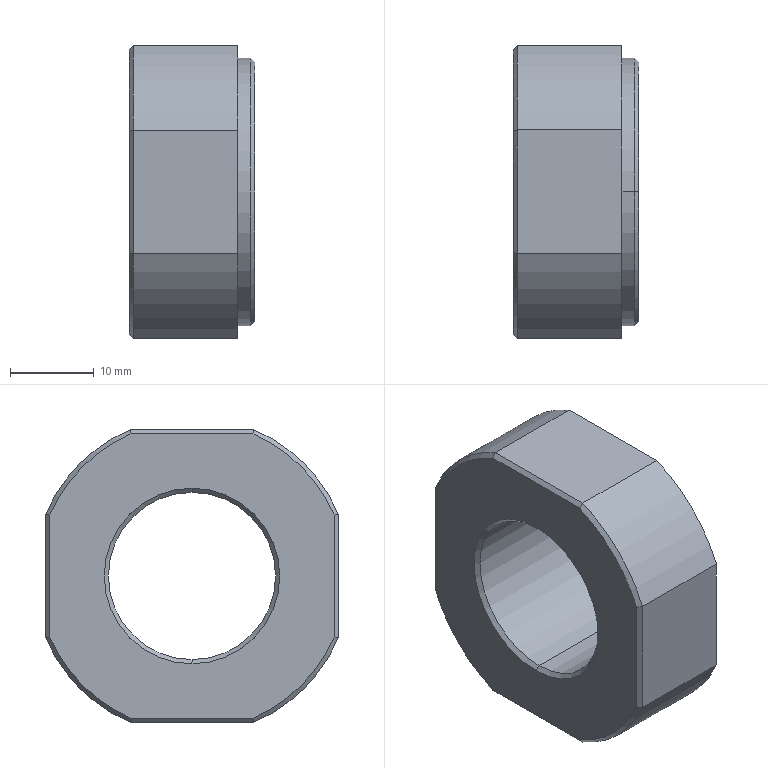Part | SolidWorks | features ICE 2, Chamfer 1, Extrusion 1 | 1 solid | 29 faces | box 15 x 35 x 35 mm | volume 10821 mm3 | plane 11 | cone 10 | cylinder 8 | commonest cylinder face diameters 38 x4 20 x2 32 x2
STEP:
#1=CARTESIAN_POINT('',(14.5,0.,10.));
#2=VERTEX_POINT('',#1);
#3=CARTESIAN_POINT('',(14.5,0.,-10.));
#4=VERTEX_POINT('',#3);
#5=CARTESIAN_POINT('',(14.5,0.,0.));
#6=DIRECTION('',(1.,0.,0.));
#7=DIRECTION('',(0.,0.,-1.));
#8=AXIS2_PLACEMENT_3D('',#5,#6,#7);
#9=CIRCLE('',#8,10.);
#10=EDGE_CURVE('',#2,#4,#9,.T.);
#11=ORIENTED_EDGE('',*,*,#10,.F.);
#12=CARTESIAN_POINT('',(15.,0.,10.5));
#13=VERTEX_POINT('',#12);
#14=CARTESIAN_POINT('',(14.5,0.,10.));
#15=DIRECTION('',(0.7071,0.,0.7071));
#16=VECTOR('',#15,1000.);
#17=LINE('',#14,#16);
#18=EDGE_CURVE('',#2,#13,#17,.T.);
#19=ORIENTED_EDGE('',*,*,#18,.T.);
#20=CARTESIAN_POINT('',(15.,0.,-10.5));
#21=VERTEX_POINT('',#20);
#22=CARTESIAN_POINT('',(15.,0.,0.));
#23=DIRECTION('',(-1.,0.,0.));
#24=DIRECTION('',(0.,0.,-1.));
#25=AXIS2_PLACEMENT_3D('',#22,#23,#24);
#26=CIRCLE('',#25,10.5);
#27=EDGE_CURVE('',#21,#13,#26,.T.);
#28=ORIENTED_EDGE('',*,*,#27,.F.);
#29=CARTESIAN_POINT('',(14.5,0.,-10.));
#30=DIRECTION('',(0.7071,0.,-0.7071));
#31=VECTOR('',#30,1000.);
#32=LINE('',#29,#31);
#33=EDGE_CURVE('',#4,#21,#32,.T.);
#34=ORIENTED_EDGE('',*,*,#33,.F.);
#35=EDGE_LOOP('',(#11,#19,#28,#34));
#36=FACE_OUTER_BOUND('',#35,.T.);
#37=CARTESIAN_POINT('',(14.5,0.,0.));
#38=DIRECTION('',(1.,0.,0.));
#39=DIRECTION('',(0.,0.,-1.));
#40=AXIS2_PLACEMENT_3D('',#37,#38,#39);
#41=CONICAL_SURFACE('',#40,10.,0.7854);
#42=ADVANCED_FACE('',(#36),#41,.F.);
#43=CARTESIAN_POINT('',(15.,0.,-15.5));
#44=VERTEX_POINT('',#43);
#45=CARTESIAN_POINT('',(15.,0.,15.5));
#46=VERTEX_POINT('',#45);
#47=CARTESIAN_POINT('',(15.,0.,0.));
#48=DIRECTION('',(1.,0.,0.));
#49=DIRECTION('',(0.,0.,-1.));
#50=AXIS2_PLACEMENT_3D('',#47,#48,#49);
#51=CIRCLE('',#50,15.5);
#52=EDGE_CURVE('',#44,#46,#51,.T.);
#53=ORIENTED_EDGE('',*,*,#52,.F.);
#54=CARTESIAN_POINT('',(14.5,0.,-16.));
#55=VERTEX_POINT('',#54);
#56=CARTESIAN_POINT('',(15.,0.,-15.5));
#57=DIRECTION('',(-0.7071,0.,-0.7071));
#58=VECTOR('',#57,1000.);
#59=LINE('',#56,#58);
#60=EDGE_CURVE('',#44,#55,#59,.T.);
#61=ORIENTED_EDGE('',*,*,#60,.T.);
#62=CARTESIAN_POINT('',(14.5,0.,16.));
#63=VERTEX_POINT('',#62);
#64=CARTESIAN_POINT('',(14.5,0.,0.));
#65=DIRECTION('',(-1.,0.,0.));
#66=DIRECTION('',(0.,0.,-1.));
#67=AXIS2_PLACEMENT_3D('',#64,#65,#66);
#68=CIRCLE('',#67,16.);
#69=EDGE_CURVE('',#63,#55,#68,.T.);
#70=ORIENTED_EDGE('',*,*,#69,.F.);
#71=CARTESIAN_POINT('',(15.,0.,15.5));
#72=DIRECTION('',(-0.7071,0.,0.7071));
#73=VECTOR('',#72,1000.);
#74=LINE('',#71,#73);
#75=EDGE_CURVE('',#46,#63,#74,.T.);
#76=ORIENTED_EDGE('',*,*,#75,.F.);
#77=EDGE_LOOP('',(#53,#61,#70,#76));
#78=FACE_OUTER_BOUND('',#77,.T.);
#79=CARTESIAN_POINT('',(15.,0.,0.));
#80=DIRECTION('',(-1.,0.,0.));
#81=DIRECTION('',(0.,0.,1.));
#82=AXIS2_PLACEMENT_3D('',#79,#80,#81);
#83=CONICAL_SURFACE('',#82,15.5,0.7854);
#84=ADVANCED_FACE('',(#78),#83,.T.);
#85=CARTESIAN_POINT('',(0.5,0.,-10.));
#86=VERTEX_POINT('',#85);
#87=CARTESIAN_POINT('',(0.5,0.,10.));
#88=VERTEX_POINT('',#87);
#89=CARTESIAN_POINT('',(0.5,0.,0.));
#90=DIRECTION('',(-1.,0.,0.));
#91=DIRECTION('',(0.,0.,-1.));
#92=AXIS2_PLACEMENT_3D('',#89,#90,#91);
#93=CIRCLE('',#92,10.);
#94=EDGE_CURVE('',#86,#88,#93,.T.);
#95=ORIENTED_EDGE('',*,*,#94,.F.);
#96=CARTESIAN_POINT('',(0.,0.,-10.5));
#97=VERTEX_POINT('',#96);
#98=CARTESIAN_POINT('',(0.,0.,-10.5));
#99=DIRECTION('',(-0.7071,0.,-0.7071));
#100=VECTOR('',#99,1000.);
#101=LINE('',#98,#100);
#102=EDGE_CURVE('',#86,#97,#101,.T.);
#103=ORIENTED_EDGE('',*,*,#102,.T.);
#104=CARTESIAN_POINT('',(0.,0.,10.5));
#105=VERTEX_POINT('',#104);
#106=CARTESIAN_POINT('',(0.,0.,0.));
#107=DIRECTION('',(1.,0.,0.));
#108=DIRECTION('',(0.,0.,-1.));
#109=AXIS2_PLACEMENT_3D('',#106,#107,#108);
#110=CIRCLE('',#109,10.5);
#111=EDGE_CURVE('',#105,#97,#110,.T.);
#112=ORIENTED_EDGE('',*,*,#111,.F.);
#113=CARTESIAN_POINT('',(0.,0.,10.5));
#114=DIRECTION('',(-0.7071,0.,0.7071));
#115=VECTOR('',#114,1000.);
#116=LINE('',#113,#115);
#117=EDGE_CURVE('',#88,#105,#116,.T.);
#118=ORIENTED_EDGE('',*,*,#117,.F.);
#119=EDGE_LOOP('',(#95,#103,#112,#118));
#120=FACE_OUTER_BOUND('',#119,.T.);
#121=CARTESIAN_POINT('',(0.,0.,0.));
#122=DIRECTION('',(-1.,0.,0.));
#123=DIRECTION('',(0.,0.,1.));
#124=AXIS2_PLACEMENT_3D('',#121,#122,#123);
#125=CONICAL_SURFACE('',#124,10.5,0.7854);
#126=ADVANCED_FACE('',(#120),#125,.F.);
#127=CARTESIAN_POINT('',(13.,0.,-16.));
#128=VERTEX_POINT('',#127);
#129=CARTESIAN_POINT('',(13.,0.,16.));
#130=VERTEX_POINT('',#129);
#131=CARTESIAN_POINT('',(13.,0.,0.));
#132=DIRECTION('',(1.,0.,0.));
#133=DIRECTION('',(0.,0.,-1.));
#134=AXIS2_PLACEMENT_3D('',#131,#132,#133);
#135=CIRCLE('',#134,16.);
#136=EDGE_CURVE('',#128,#130,#135,.T.);
#137=ORIENTED_EDGE('',*,*,#136,.T.);
#138=CARTESIAN_POINT('',(13.,0.,16.));
#139=DIRECTION('',(1.,0.,0.));
#140=VECTOR('',#139,1000.);
#141=LINE('',#138,#140);
#142=EDGE_CURVE('',#130,#63,#141,.T.);
#143=ORIENTED_EDGE('',*,*,#142,.T.);
#144=ORIENTED_EDGE('',*,*,#69,.T.);
#145=CARTESIAN_POINT('',(13.,0.,-16.));
#146=DIRECTION('',(1.,0.,0.));
#147=VECTOR('',#146,1000.);
#148=LINE('',#145,#147);
#149=EDGE_CURVE('',#128,#55,#148,.T.);
#150=ORIENTED_EDGE('',*,*,#149,.F.);
#151=EDGE_LOOP('',(#137,#143,#144,#150));
#152=FACE_OUTER_BOUND('',#151,.T.);
#153=CARTESIAN_POINT('',(13.,0.,0.));
#154=DIRECTION('',(1.,0.,0.));
#155=DIRECTION('',(0.,0.,-1.));
#156=AXIS2_PLACEMENT_3D('',#153,#154,#155);
#157=CYLINDRICAL_SURFACE('',#156,16.);
#158=ADVANCED_FACE('',(#152),#157,.T.);
#159=ORIENTED_EDGE('',*,*,#10,.T.);
#160=CARTESIAN_POINT('',(15.,0.,-10.));
#161=DIRECTION('',(-1.,0.,0.));
#162=VECTOR('',#161,1000.);
#163=LINE('',#160,#162);
#164=EDGE_CURVE('',#4,#86,#163,.T.);
#165=ORIENTED_EDGE('',*,*,#164,.T.);
#166=ORIENTED_EDGE('',*,*,#94,.T.);
#167=CARTESIAN_POINT('',(15.,0.,10.));
#168=DIRECTION('',(-1.,0.,0.));
#169=VECTOR('',#168,1000.);
#170=LINE('',#167,#169);
#171=EDGE_CURVE('',#2,#88,#170,.T.);
#172=ORIENTED_EDGE('',*,*,#171,.F.);
#173=EDGE_LOOP('',(#159,#165,#166,#172));
#174=FACE_OUTER_BOUND('',#173,.T.);
#175=CARTESIAN_POINT('',(15.,0.,0.));
#176=DIRECTION('',(-1.,0.,0.));
#177=DIRECTION('',(0.,0.,1.));
#178=AXIS2_PLACEMENT_3D('',#175,#176,#177);
#179=CYLINDRICAL_SURFACE('',#178,10.);
#180=ADVANCED_FACE('',(#174),#179,.F.);
#181=CARTESIAN_POINT('',(0.5,17.5,7.399));
#182=VERTEX_POINT('',#181);
#183=CARTESIAN_POINT('',(13.,17.5,7.399));
#184=VERTEX_POINT('',#183);
#185=CARTESIAN_POINT('',(15.,17.5,7.399));
#186=DIRECTION('',(1.,0.,0.));
#187=VECTOR('',#186,1000.);
#188=LINE('',#185,#187);
#189=EDGE_CURVE('',#182,#184,#188,.T.);
#190=ORIENTED_EDGE('',*,*,#189,.F.);
#191=CARTESIAN_POINT('',(0.5,7.399,17.5));
#192=VERTEX_POINT('',#191);
#193=CARTESIAN_POINT('',(0.5,0.,0.));
#194=DIRECTION('',(1.,0.,0.));
#195=DIRECTION('',(0.,0.,-1.));
#196=AXIS2_PLACEMENT_3D('',#193,#194,#195);
#197=CIRCLE('',#196,19.);
#198=EDGE_CURVE('',#182,#192,#197,.T.);
#199=ORIENTED_EDGE('',*,*,#198,.T.);
#200=CARTESIAN_POINT('',(13.,7.399,17.5));
#201=VERTEX_POINT('',#200);
#202=CARTESIAN_POINT('',(15.,7.399,17.5));
#203=DIRECTION('',(-1.,0.,0.));
#204=VECTOR('',#203,1000.);
#205=LINE('',#202,#204);
#206=EDGE_CURVE('',#201,#192,#205,.T.);
#207=ORIENTED_EDGE('',*,*,#206,.F.);
#208=CARTESIAN_POINT('',(13.,0.,0.));
#209=DIRECTION('',(1.,0.,0.));
#210=DIRECTION('',(0.,0.,-1.));
#211=AXIS2_PLACEMENT_3D('',#208,#209,#210);
#212=CIRCLE('',#211,19.);
#213=EDGE_CURVE('',#184,#201,#212,.T.);
#214=ORIENTED_EDGE('',*,*,#213,.F.);
#215=EDGE_LOOP('',(#190,#199,#207,#214));
#216=FACE_OUTER_BOUND('',#215,.T.);
#217=CARTESIAN_POINT('',(15.,0.,0.));
#218=DIRECTION('',(-1.,0.,0.));
#219=DIRECTION('',(0.,0.,1.));
#220=AXIS2_PLACEMENT_3D('',#217,#218,#219);
#221=CYLINDRICAL_SURFACE('',#220,19.);
#222=ADVANCED_FACE('',(#216),#221,.T.);
#223=CARTESIAN_POINT('',(0.5,-7.399,17.5));
#224=VERTEX_POINT('',#223);
#225=CARTESIAN_POINT('',(13.,-7.399,17.5));
#226=VERTEX_POINT('',#225);
#227=CARTESIAN_POINT('',(15.,-7.399,17.5));
#228=DIRECTION('',(1.,0.,0.));
#229=VECTOR('',#228,1000.);
#230=LINE('',#227,#229);
#231=EDGE_CURVE('',#224,#226,#230,.T.);
#232=ORIENTED_EDGE('',*,*,#231,.F.);
#233=CARTESIAN_POINT('',(0.5,-17.5,7.399));
#234=VERTEX_POINT('',#233);
#235=CARTESIAN_POINT('',(0.5,0.,0.));
#236=DIRECTION('',(1.,0.,0.));
#237=DIRECTION('',(0.,0.,-1.));
#238=AXIS2_PLACEMENT_3D('',#235,#236,#237);
#239=CIRCLE('',#238,19.);
#240=EDGE_CURVE('',#224,#234,#239,.T.);
#241=ORIENTED_EDGE('',*,*,#240,.T.);
#242=CARTESIAN_POINT('',(13.,-17.5,7.399));
#243=VERTEX_POINT('',#242);
#244=CARTESIAN_POINT('',(15.,-17.5,7.399));
#245=DIRECTION('',(-1.,0.,0.));
#246=VECTOR('',#245,1000.);
#247=LINE('',#244,#246);
#248=EDGE_CURVE('',#243,#234,#247,.T.);
#249=ORIENTED_EDGE('',*,*,#248,.F.);
#250=CARTESIAN_POINT('',(13.,0.,0.));
#251=DIRECTION('',(1.,0.,0.));
#252=DIRECTION('',(0.,0.,-1.));
#253=AXIS2_PLACEMENT_3D('',#250,#251,#252);
#254=CIRCLE('',#253,19.);
#255=EDGE_CURVE('',#226,#243,#254,.T.);
#256=ORIENTED_EDGE('',*,*,#255,.F.);
#257=EDGE_LOOP('',(#232,#241,#249,#256));
#258=FACE_OUTER_BOUND('',#257,.T.);
#259=CARTESIAN_POINT('',(15.,0.,0.));
#260=DIRECTION('',(-1.,0.,0.));
#261=DIRECTION('',(0.,0.,1.));
#262=AXIS2_PLACEMENT_3D('',#259,#260,#261);
#263=CYLINDRICAL_SURFACE('',#262,19.);
#264=ADVANCED_FACE('',(#258),#263,.T.);
#265=CARTESIAN_POINT('',(0.5,-17.5,-7.399));
#266=VERTEX_POINT('',#265);
#267=CARTESIAN_POINT('',(13.,-17.5,-7.399));
#268=VERTEX_POINT('',#267);
#269=CARTESIAN_POINT('',(15.,-17.5,-7.399));
#270=DIRECTION('',(1.,0.,0.));
#271=VECTOR('',#270,1000.);
#272=LINE('',#269,#271);
#273=EDGE_CURVE('',#266,#268,#272,.T.);
#274=ORIENTED_EDGE('',*,*,#273,.F.);
#275=CARTESIAN_POINT('',(0.5,-7.399,-17.5));
#276=VERTEX_POINT('',#275);
#277=CARTESIAN_POINT('',(0.5,0.,0.));
#278=DIRECTION('',(1.,0.,0.));
#279=DIRECTION('',(0.,0.,-1.));
#280=AXIS2_PLACEMENT_3D('',#277,#278,#279);
#281=CIRCLE('',#280,19.);
#282=EDGE_CURVE('',#266,#276,#281,.T.);
#283=ORIENTED_EDGE('',*,*,#282,.T.);
#284=CARTESIAN_POINT('',(13.,-7.399,-17.5));
#285=VERTEX_POINT('',#284);
#286=CARTESIAN_POINT('',(15.,-7.399,-17.5));
#287=DIRECTION('',(-1.,0.,0.));
#288=VECTOR('',#287,1000.);
#289=LINE('',#286,#288);
#290=EDGE_CURVE('',#285,#276,#289,.T.);
#291=ORIENTED_EDGE('',*,*,#290,.F.);
#292=CARTESIAN_POINT('',(13.,0.,0.));
#293=DIRECTION('',(1.,0.,0.));
#294=DIRECTION('',(0.,0.,-1.));
#295=AXIS2_PLACEMENT_3D('',#292,#293,#294);
#296=CIRCLE('',#295,19.);
#297=EDGE_CURVE('',#268,#285,#296,.T.);
#298=ORIENTED_EDGE('',*,*,#297,.F.);
#299=EDGE_LOOP('',(#274,#283,#291,#298));
#300=FACE_OUTER_BOUND('',#299,.T.);
#301=CARTESIAN_POINT('',(15.,0.,0.));
#302=DIRECTION('',(-1.,0.,0.));
#303=DIRECTION('',(0.,0.,1.));
#304=AXIS2_PLACEMENT_3D('',#301,#302,#303);
#305=CYLINDRICAL_SURFACE('',#304,19.);
#306=ADVANCED_FACE('',(#300),#305,.T.);
#307=CARTESIAN_POINT('',(0.5,7.399,-17.5));
#308=VERTEX_POINT('',#307);
#309=CARTESIAN_POINT('',(13.,7.399,-17.5));
#310=VERTEX_POINT('',#309);
#311=CARTESIAN_POINT('',(15.,7.399,-17.5));
#312=DIRECTION('',(1.,0.,0.));
#313=VECTOR('',#312,1000.);
#314=LINE('',#311,#313);
#315=EDGE_CURVE('',#308,#310,#314,.T.);
#316=ORIENTED_EDGE('',*,*,#315,.F.);
#317=CARTESIAN_POINT('',(0.5,17.5,-7.399));
#318=VERTEX_POINT('',#317);
#319=CARTESIAN_POINT('',(0.5,0.,0.));
#320=DIRECTION('',(1.,0.,0.));
#321=DIRECTION('',(0.,0.,-1.));
#322=AXIS2_PLACEMENT_3D('',#319,#320,#321);
#323=CIRCLE('',#322,19.);
#324=EDGE_CURVE('',#308,#318,#323,.T.);
#325=ORIENTED_EDGE('',*,*,#324,.T.);
#326=CARTESIAN_POINT('',(13.,17.5,-7.399));
#327=VERTEX_POINT('',#326);
#328=CARTESIAN_POINT('',(15.,17.5,-7.399));
#329=DIRECTION('',(-1.,0.,0.));
#330=VECTOR('',#329,1000.);
#331=LINE('',#328,#330);
#332=EDGE_CURVE('',#327,#318,#331,.T.);
#333=ORIENTED_EDGE('',*,*,#332,.F.);
#334=CARTESIAN_POINT('',(13.,0.,0.));
#335=DIRECTION('',(1.,0.,0.));
#336=DIRECTION('',(0.,0.,-1.));
#337=AXIS2_PLACEMENT_3D('',#334,#335,#336);
#338=CIRCLE('',#337,19.);
#339=EDGE_CURVE('',#310,#327,#338,.T.);
#340=ORIENTED_EDGE('',*,*,#339,.F.);
#341=EDGE_LOOP('',(#316,#325,#333,#340));
#342=FACE_OUTER_BOUND('',#341,.T.);
#343=CARTESIAN_POINT('',(15.,0.,0.));
#344=DIRECTION('',(-1.,0.,0.));
#345=DIRECTION('',(0.,0.,1.));
#346=AXIS2_PLACEMENT_3D('',#343,#344,#345);
#347=CYLINDRICAL_SURFACE('',#346,19.);
#348=ADVANCED_FACE('',(#342),#347,.T.);
#349=CARTESIAN_POINT('',(0.,-17.,-7.297));
#350=VERTEX_POINT('',#349);
#351=CARTESIAN_POINT('',(0.,-17.,7.297));
#352=VERTEX_POINT('',#351);
#353=CARTESIAN_POINT('',(0.,-17.,7.399));
#354=DIRECTION('',(0.,0.,1.));
#355=VECTOR('',#354,1000.);
#356=LINE('',#353,#355);
#357=EDGE_CURVE('',#350,#352,#356,.T.);
#358=ORIENTED_EDGE('',*,*,#357,.T.);
#359=CARTESIAN_POINT('',(0.,-7.297,17.));
#360=VERTEX_POINT('',#359);
#361=CARTESIAN_POINT('',(0.,0.,0.));
#362=DIRECTION('',(-1.,0.,0.));
#363=DIRECTION('',(0.,0.,-1.));
#364=AXIS2_PLACEMENT_3D('',#361,#362,#363);
#365=CIRCLE('',#364,18.5);
#366=EDGE_CURVE('',#352,#360,#365,.T.);
#367=ORIENTED_EDGE('',*,*,#366,.T.);
#368=CARTESIAN_POINT('',(0.,7.297,17.));
#369=VERTEX_POINT('',#368);
#370=CARTESIAN_POINT('',(0.,7.399,17.));
#371=DIRECTION('',(0.,1.,0.));
#372=VECTOR('',#371,1000.);
#373=LINE('',#370,#372);
#374=EDGE_CURVE('',#360,#369,#373,.T.);
#375=ORIENTED_EDGE('',*,*,#374,.T.);
#376=CARTESIAN_POINT('',(0.,17.,7.297));
#377=VERTEX_POINT('',#376);
#378=CARTESIAN_POINT('',(0.,0.,0.));
#379=DIRECTION('',(-1.,0.,0.));
#380=DIRECTION('',(0.,0.,-1.));
#381=AXIS2_PLACEMENT_3D('',#378,#379,#380);
#382=CIRCLE('',#381,18.5);
#383=EDGE_CURVE('',#369,#377,#382,.T.);
#384=ORIENTED_EDGE('',*,*,#383,.T.);
#385=CARTESIAN_POINT('',(0.,17.,-7.297));
#386=VERTEX_POINT('',#385);
#387=CARTESIAN_POINT('',(0.,17.,-7.399));
#388=DIRECTION('',(0.,0.,-1.));
#389=VECTOR('',#388,1000.);
#390=LINE('',#387,#389);
#391=EDGE_CURVE('',#377,#386,#390,.T.);
#392=ORIENTED_EDGE('',*,*,#391,.T.);
#393=CARTESIAN_POINT('',(0.,7.297,-17.));
#394=VERTEX_POINT('',#393);
#395=CARTESIAN_POINT('',(0.,0.,0.));
#396=DIRECTION('',(-1.,0.,0.));
#397=DIRECTION('',(0.,0.,-1.));
#398=AXIS2_PLACEMENT_3D('',#395,#396,#397);
#399=CIRCLE('',#398,18.5);
#400=EDGE_CURVE('',#386,#394,#399,.T.);
#401=ORIENTED_EDGE('',*,*,#400,.T.);
#402=CARTESIAN_POINT('',(0.,-7.297,-17.));
#403=VERTEX_POINT('',#402);
#404=CARTESIAN_POINT('',(0.,-7.399,-17.));
#405=DIRECTION('',(0.,-1.,0.));
#406=VECTOR('',#405,1000.);
#407=LINE('',#404,#406);
#408=EDGE_CURVE('',#394,#403,#407,.T.);
#409=ORIENTED_EDGE('',*,*,#408,.T.);
#410=CARTESIAN_POINT('',(0.,0.,0.));
#411=DIRECTION('',(-1.,0.,0.));
#412=DIRECTION('',(0.,0.,-1.));
#413=AXIS2_PLACEMENT_3D('',#410,#411,#412);
#414=CIRCLE('',#413,18.5);
#415=EDGE_CURVE('',#403,#350,#414,.T.);
#416=ORIENTED_EDGE('',*,*,#415,.T.);
#417=EDGE_LOOP('',(#358,#367,#375,#384,#392,#401,#409,#416));
#418=FACE_OUTER_BOUND('',#417,.T.);
#419=ORIENTED_EDGE('',*,*,#111,.T.);
#420=CARTESIAN_POINT('',(0.,0.,0.));
#421=DIRECTION('',(1.,0.,0.));
#422=DIRECTION('',(0.,0.,-1.));
#423=AXIS2_PLACEMENT_3D('',#420,#421,#422);
#424=CIRCLE('',#423,10.5);
#425=EDGE_CURVE('',#97,#105,#424,.T.);
#426=ORIENTED_EDGE('',*,*,#425,.T.);
#427=EDGE_LOOP('',(#419,#426));
#428=FACE_BOUND('',#427,.T.);
#429=CARTESIAN_POINT('',(0.,0.,0.));
#430=DIRECTION('',(1.,0.,0.));
#431=DIRECTION('',(0.,0.,-1.));
#432=AXIS2_PLACEMENT_3D('',#429,#430,#431);
#433=PLANE('',#432);
#434=ADVANCED_FACE('',(#418,#428),#433,.F.);
#435=ORIENTED_EDGE('',*,*,#136,.F.);
#436=CARTESIAN_POINT('',(13.,0.,0.));
#437=DIRECTION('',(1.,0.,0.));
#438=DIRECTION('',(0.,0.,-1.));
#439=AXIS2_PLACEMENT_3D('',#436,#437,#438);
#440=CIRCLE('',#439,16.);
#441=EDGE_CURVE('',#130,#128,#440,.T.);
#442=ORIENTED_EDGE('',*,*,#441,.F.);
#443=EDGE_LOOP('',(#435,#442));
#444=FACE_BOUND('',#443,.T.);
#445=ORIENTED_EDGE('',*,*,#213,.T.);
#446=CARTESIAN_POINT('',(13.,0.,17.5));
#447=DIRECTION('',(0.,-1.,0.));
#448=VECTOR('',#447,1000.);
#449=LINE('',#446,#448);
#450=EDGE_CURVE('',#201,#226,#449,.T.);
#451=ORIENTED_EDGE('',*,*,#450,.T.);
#452=ORIENTED_EDGE('',*,*,#255,.T.);
#453=CARTESIAN_POINT('',(13.,-17.5,0.));
#454=DIRECTION('',(0.,0.,-1.));
#455=VECTOR('',#454,1000.);
#456=LINE('',#453,#455);
#457=EDGE_CURVE('',#243,#268,#456,.T.);
#458=ORIENTED_EDGE('',*,*,#457,.T.);
#459=ORIENTED_EDGE('',*,*,#297,.T.);
#460=CARTESIAN_POINT('',(13.,0.,-17.5));
#461=DIRECTION('',(0.,1.,0.));
#462=VECTOR('',#461,1000.);
#463=LINE('',#460,#462);
#464=EDGE_CURVE('',#285,#310,#463,.T.);
#465=ORIENTED_EDGE('',*,*,#464,.T.);
#466=ORIENTED_EDGE('',*,*,#339,.T.);
#467=CARTESIAN_POINT('',(13.,17.5,0.));
#468=DIRECTION('',(0.,0.,1.));
#469=VECTOR('',#468,1000.);
#470=LINE('',#467,#469);
#471=EDGE_CURVE('',#327,#184,#470,.T.);
#472=ORIENTED_EDGE('',*,*,#471,.T.);
#473=EDGE_LOOP('',(#445,#451,#452,#458,#459,#465,#466,#472));
#474=FACE_OUTER_BOUND('',#473,.T.);
#475=CARTESIAN_POINT('',(13.,0.,0.));
#476=DIRECTION('',(1.,0.,0.));
#477=DIRECTION('',(0.,0.,-1.));
#478=AXIS2_PLACEMENT_3D('',#475,#476,#477);
#479=PLANE('',#478);
#480=ADVANCED_FACE('',(#444,#474),#479,.T.);
#481=CARTESIAN_POINT('',(15.,0.,0.));
#482=DIRECTION('',(1.,0.,0.));
#483=DIRECTION('',(0.,0.,-1.));
#484=AXIS2_PLACEMENT_3D('',#481,#482,#483);
#485=CIRCLE('',#484,15.5);
#486=EDGE_CURVE('',#46,#44,#485,.T.);
#487=ORIENTED_EDGE('',*,*,#486,.T.);
#488=ORIENTED_EDGE('',*,*,#52,.T.);
#489=EDGE_LOOP('',(#487,#488));
#490=FACE_OUTER_BOUND('',#489,.T.);
#491=ORIENTED_EDGE('',*,*,#27,.T.);
#492=CARTESIAN_POINT('',(15.,0.,0.));
#493=DIRECTION('',(-1.,0.,0.));
#494=DIRECTION('',(0.,0.,-1.));
#495=AXIS2_PLACEMENT_3D('',#492,#493,#494);
#496=CIRCLE('',#495,10.5);
#497=EDGE_CURVE('',#13,#21,#496,.T.);
#498=ORIENTED_EDGE('',*,*,#497,.T.);
#499=EDGE_LOOP('',(#491,#498));
#500=FACE_BOUND('',#499,.T.);
#501=CARTESIAN_POINT('',(15.,0.,0.));
#502=DIRECTION('',(1.,0.,0.));
#503=DIRECTION('',(0.,0.,-1.));
#504=AXIS2_PLACEMENT_3D('',#501,#502,#503);
#505=PLANE('',#504);
#506=ADVANCED_FACE('',(#490,#500),#505,.T.);
#507=ORIENTED_EDGE('',*,*,#164,.F.);
#508=CARTESIAN_POINT('',(14.5,0.,0.));
#509=DIRECTION('',(1.,0.,0.));
#510=DIRECTION('',(0.,0.,-1.));
#511=AXIS2_PLACEMENT_3D('',#508,#509,#510);
#512=CIRCLE('',#511,10.);
#513=EDGE_CURVE('',#4,#2,#512,.T.);
#514=ORIENTED_EDGE('',*,*,#513,.T.);
#515=ORIENTED_EDGE('',*,*,#171,.T.);
#516=CARTESIAN_POINT('',(0.5,0.,0.));
#517=DIRECTION('',(-1.,0.,0.));
#518=DIRECTION('',(0.,0.,-1.));
#519=AXIS2_PLACEMENT_3D('',#516,#517,#518);
#520=CIRCLE('',#519,10.);
#521=EDGE_CURVE('',#88,#86,#520,.T.);
#522=ORIENTED_EDGE('',*,*,#521,.T.);
#523=EDGE_LOOP('',(#507,#514,#515,#522));
#524=FACE_OUTER_BOUND('',#523,.T.);
#525=CARTESIAN_POINT('',(15.,0.,0.));
#526=DIRECTION('',(-1.,0.,0.));
#527=DIRECTION('',(0.,0.,1.));
#528=AXIS2_PLACEMENT_3D('',#525,#526,#527);
#529=CYLINDRICAL_SURFACE('',#528,10.);
#530=ADVANCED_FACE('',(#524),#529,.F.);
#531=ORIENTED_EDGE('',*,*,#142,.F.);
#532=ORIENTED_EDGE('',*,*,#441,.T.);
#533=ORIENTED_EDGE('',*,*,#149,.T.);
#534=CARTESIAN_POINT('',(14.5,0.,0.));
#535=DIRECTION('',(-1.,0.,0.));
#536=DIRECTION('',(0.,0.,-1.));
#537=AXIS2_PLACEMENT_3D('',#534,#535,#536);
#538=CIRCLE('',#537,16.);
#539=EDGE_CURVE('',#55,#63,#538,.T.);
#540=ORIENTED_EDGE('',*,*,#539,.T.);
#541=EDGE_LOOP('',(#531,#532,#533,#540));
#542=FACE_OUTER_BOUND('',#541,.T.);
#543=CARTESIAN_POINT('',(13.,0.,0.));
#544=DIRECTION('',(1.,0.,0.));
#545=DIRECTION('',(0.,0.,-1.));
#546=AXIS2_PLACEMENT_3D('',#543,#544,#545);
#547=CYLINDRICAL_SURFACE('',#546,16.);
#548=ADVANCED_FACE('',(#542),#547,.T.);
#549=ORIENTED_EDGE('',*,*,#332,.T.);
#550=CARTESIAN_POINT('',(0.5,17.5,7.399));
#551=DIRECTION('',(0.,0.,1.));
#552=VECTOR('',#551,1000.);
#553=LINE('',#550,#552);
#554=EDGE_CURVE('',#318,#182,#553,.T.);
#555=ORIENTED_EDGE('',*,*,#554,.T.);
#556=ORIENTED_EDGE('',*,*,#189,.T.);
#557=ORIENTED_EDGE('',*,*,#471,.F.);
#558=EDGE_LOOP('',(#549,#555,#556,#557));
#559=FACE_OUTER_BOUND('',#558,.T.);
#560=CARTESIAN_POINT('',(15.,17.5,-17.5));
#561=DIRECTION('',(0.,1.,0.));
#562=DIRECTION('',(0.,0.,1.));
#563=AXIS2_PLACEMENT_3D('',#560,#561,#562);
#564=PLANE('',#563);
#565=ADVANCED_FACE('',(#559),#564,.T.);
#566=ORIENTED_EDGE('',*,*,#290,.T.);
#567=CARTESIAN_POINT('',(0.5,7.399,-17.5));
#568=DIRECTION('',(0.,1.,0.));
#569=VECTOR('',#568,1000.);
#570=LINE('',#567,#569);
#571=EDGE_CURVE('',#276,#308,#570,.T.);
#572=ORIENTED_EDGE('',*,*,#571,.T.);
#573=ORIENTED_EDGE('',*,*,#315,.T.);
#574=ORIENTED_EDGE('',*,*,#464,.F.);
#575=EDGE_LOOP('',(#566,#572,#573,#574));
#576=FACE_OUTER_BOUND('',#575,.T.);
#577=CARTESIAN_POINT('',(15.,-17.5,-17.5));
#578=DIRECTION('',(0.,0.,-1.));
#579=DIRECTION('',(-1.,0.,0.));
#580=AXIS2_PLACEMENT_3D('',#577,#578,#579);
#581=PLANE('',#580);
#582=ADVANCED_FACE('',(#576),#581,.T.);
#583=ORIENTED_EDGE('',*,*,#248,.T.);
#584=CARTESIAN_POINT('',(0.5,-17.5,-7.399));
#585=DIRECTION('',(0.,0.,-1.));
#586=VECTOR('',#585,1000.);
#587=LINE('',#584,#586);
#588=EDGE_CURVE('',#234,#266,#587,.T.);
#589=ORIENTED_EDGE('',*,*,#588,.T.);
#590=ORIENTED_EDGE('',*,*,#273,.T.);
#591=ORIENTED_EDGE('',*,*,#457,.F.);
#592=EDGE_LOOP('',(#583,#589,#590,#591));
#593=FACE_OUTER_BOUND('',#592,.T.);
#594=CARTESIAN_POINT('',(15.,-17.5,-17.5));
#595=DIRECTION('',(0.,-1.,0.));
#596=DIRECTION('',(0.,0.,-1.));
#597=AXIS2_PLACEMENT_3D('',#594,#595,#596);
#598=PLANE('',#597);
#599=ADVANCED_FACE('',(#593),#598,.T.);
#600=ORIENTED_EDGE('',*,*,#206,.T.);
#601=CARTESIAN_POINT('',(0.5,-7.399,17.5));
#602=DIRECTION('',(0.,-1.,0.));
#603=VECTOR('',#602,1000.);
#604=LINE('',#601,#603);
#605=EDGE_CURVE('',#192,#224,#604,.T.);
#606=ORIENTED_EDGE('',*,*,#605,.T.);
#607=ORIENTED_EDGE('',*,*,#231,.T.);
#608=ORIENTED_EDGE('',*,*,#450,.F.);
#609=EDGE_LOOP('',(#600,#606,#607,#608));
#610=FACE_OUTER_BOUND('',#609,.T.);
#611=CARTESIAN_POINT('',(15.,-17.5,17.5));
#612=DIRECTION('',(0.,0.,1.));
#613=DIRECTION('',(1.,0.,0.));
#614=AXIS2_PLACEMENT_3D('',#611,#612,#613);
#615=PLANE('',#614);
#616=ADVANCED_FACE('',(#610),#615,.T.);
#617=CARTESIAN_POINT('',(0.,7.297,-17.));
#618=CARTESIAN_POINT('',(0.1666,7.332,-17.167));
#619=CARTESIAN_POINT('',(0.3333,7.366,-17.333));
#620=CARTESIAN_POINT('',(0.5,7.399,-17.5));
#621=B_SPLINE_CURVE_WITH_KNOTS('',3,(#617,#618,#619,#620),.UNSPECIFIED.,.F.,.F.,(4,4),(0.,0.0007144),.UNSPECIFIED.);
#622=EDGE_CURVE('',#394,#308,#621,.T.);
#623=ORIENTED_EDGE('',*,*,#622,.F.);
#624=ORIENTED_EDGE('',*,*,#400,.F.);
#625=CARTESIAN_POINT('',(0.5,17.5,-7.399));
#626=CARTESIAN_POINT('',(0.3333,17.333,-7.366));
#627=CARTESIAN_POINT('',(0.1666,17.167,-7.332));
#628=CARTESIAN_POINT('',(0.,17.,-7.297));
#629=B_SPLINE_CURVE_WITH_KNOTS('',3,(#625,#626,#627,#628),.UNSPECIFIED.,.F.,.F.,(4,4),(0.,0.0007144),.UNSPECIFIED.);
#630=EDGE_CURVE('',#318,#386,#629,.T.);
#631=ORIENTED_EDGE('',*,*,#630,.F.);
#632=ORIENTED_EDGE('',*,*,#324,.F.);
#633=EDGE_LOOP('',(#623,#624,#631,#632));
#634=FACE_OUTER_BOUND('',#633,.T.);
#635=CARTESIAN_POINT('',(0.5,0.,0.));
#636=DIRECTION('',(1.,0.,0.));
#637=DIRECTION('',(0.,0.,-1.));
#638=AXIS2_PLACEMENT_3D('',#635,#636,#637);
#639=CONICAL_SURFACE('',#638,19.,0.7854);
#640=ADVANCED_FACE('',(#634),#639,.T.);
#641=ORIENTED_EDGE('',*,*,#630,.T.);
#642=ORIENTED_EDGE('',*,*,#391,.F.);
#643=CARTESIAN_POINT('',(0.5,17.5,7.399));
#644=CARTESIAN_POINT('',(0.3333,17.333,7.366));
#645=CARTESIAN_POINT('',(0.1666,17.167,7.332));
#646=CARTESIAN_POINT('',(0.,17.,7.297));
#647=B_SPLINE_CURVE_WITH_KNOTS('',3,(#643,#644,#645,#646),.UNSPECIFIED.,.F.,.F.,(4,4),(0.,0.0007144),.UNSPECIFIED.);
#648=EDGE_CURVE('',#182,#377,#647,.T.);
#649=ORIENTED_EDGE('',*,*,#648,.F.);
#650=ORIENTED_EDGE('',*,*,#554,.F.);
#651=EDGE_LOOP('',(#641,#642,#649,#650));
#652=FACE_OUTER_BOUND('',#651,.T.);
#653=CARTESIAN_POINT('',(0.,17.,0.));
#654=DIRECTION('',(-0.7071,0.7071,0.));
#655=DIRECTION('',(0.,0.,1.));
#656=AXIS2_PLACEMENT_3D('',#653,#654,#655);
#657=PLANE('',#656);
#658=ADVANCED_FACE('',(#652),#657,.T.);
#659=ORIENTED_EDGE('',*,*,#622,.T.);
#660=ORIENTED_EDGE('',*,*,#571,.F.);
#661=CARTESIAN_POINT('',(0.,-7.297,-17.));
#662=CARTESIAN_POINT('',(0.1666,-7.332,-17.167));
#663=CARTESIAN_POINT('',(0.3333,-7.366,-17.333));
#664=CARTESIAN_POINT('',(0.5,-7.399,-17.5));
#665=B_SPLINE_CURVE_WITH_KNOTS('',3,(#661,#662,#663,#664),.UNSPECIFIED.,.F.,.F.,(4,4),(0.,0.0007144),.UNSPECIFIED.);
#666=EDGE_CURVE('',#403,#276,#665,.T.);
#667=ORIENTED_EDGE('',*,*,#666,.F.);
#668=ORIENTED_EDGE('',*,*,#408,.F.);
#669=EDGE_LOOP('',(#659,#660,#667,#668));
#670=FACE_OUTER_BOUND('',#669,.T.);
#671=CARTESIAN_POINT('',(0.,0.,-17.));
#672=DIRECTION('',(-0.7071,0.,-0.7071));
#673=DIRECTION('',(0.,1.,0.));
#674=AXIS2_PLACEMENT_3D('',#671,#672,#673);
#675=PLANE('',#674);
#676=ADVANCED_FACE('',(#670),#675,.T.);
#677=ORIENTED_EDGE('',*,*,#648,.T.);
#678=ORIENTED_EDGE('',*,*,#383,.F.);
#679=CARTESIAN_POINT('',(0.5,7.399,17.5));
#680=CARTESIAN_POINT('',(0.3333,7.366,17.333));
#681=CARTESIAN_POINT('',(0.1666,7.332,17.167));
#682=CARTESIAN_POINT('',(0.,7.297,17.));
#683=B_SPLINE_CURVE_WITH_KNOTS('',3,(#679,#680,#681,#682),.UNSPECIFIED.,.F.,.F.,(4,4),(0.,0.0007144),.UNSPECIFIED.);
#684=EDGE_CURVE('',#192,#369,#683,.T.);
#685=ORIENTED_EDGE('',*,*,#684,.F.);
#686=ORIENTED_EDGE('',*,*,#198,.F.);
#687=EDGE_LOOP('',(#677,#678,#685,#686));
#688=FACE_OUTER_BOUND('',#687,.T.);
#689=CARTESIAN_POINT('',(0.5,0.,0.));
#690=DIRECTION('',(1.,0.,0.));
#691=DIRECTION('',(0.,0.,-1.));
#692=AXIS2_PLACEMENT_3D('',#689,#690,#691);
#693=CONICAL_SURFACE('',#692,19.,0.7854);
#694=ADVANCED_FACE('',(#688),#693,.T.);
#695=ORIENTED_EDGE('',*,*,#666,.T.);
#696=ORIENTED_EDGE('',*,*,#282,.F.);
#697=CARTESIAN_POINT('',(0.,-17.,-7.297));
#698=CARTESIAN_POINT('',(0.1666,-17.167,-7.332));
#699=CARTESIAN_POINT('',(0.3333,-17.333,-7.366));
#700=CARTESIAN_POINT('',(0.5,-17.5,-7.399));
#701=B_SPLINE_CURVE_WITH_KNOTS('',3,(#697,#698,#699,#700),.UNSPECIFIED.,.F.,.F.,(4,4),(0.,0.0007144),.UNSPECIFIED.);
#702=EDGE_CURVE('',#350,#266,#701,.T.);
#703=ORIENTED_EDGE('',*,*,#702,.F.);
#704=ORIENTED_EDGE('',*,*,#415,.F.);
#705=EDGE_LOOP('',(#695,#696,#703,#704));
#706=FACE_OUTER_BOUND('',#705,.T.);
#707=CARTESIAN_POINT('',(0.5,0.,0.));
#708=DIRECTION('',(1.,0.,0.));
#709=DIRECTION('',(0.,0.,-1.));
#710=AXIS2_PLACEMENT_3D('',#707,#708,#709);
#711=CONICAL_SURFACE('',#710,19.,0.7854);
#712=ADVANCED_FACE('',(#706),#711,.T.);
#713=ORIENTED_EDGE('',*,*,#684,.T.);
#714=ORIENTED_EDGE('',*,*,#374,.F.);
#715=CARTESIAN_POINT('',(0.5,-7.399,17.5));
#716=CARTESIAN_POINT('',(0.3333,-7.366,17.333));
#717=CARTESIAN_POINT('',(0.1666,-7.332,17.167));
#718=CARTESIAN_POINT('',(0.,-7.297,17.));
#719=B_SPLINE_CURVE_WITH_KNOTS('',3,(#715,#716,#717,#718),.UNSPECIFIED.,.F.,.F.,(4,4),(0.,0.0007144),.UNSPECIFIED.);
#720=EDGE_CURVE('',#224,#360,#719,.T.);
#721=ORIENTED_EDGE('',*,*,#720,.F.);
#722=ORIENTED_EDGE('',*,*,#605,.F.);
#723=EDGE_LOOP('',(#713,#714,#721,#722));
#724=FACE_OUTER_BOUND('',#723,.T.);
#725=CARTESIAN_POINT('',(0.,0.,17.));
#726=DIRECTION('',(-0.7071,0.,0.7071));
#727=DIRECTION('',(0.,-1.,0.));
#728=AXIS2_PLACEMENT_3D('',#725,#726,#727);
#729=PLANE('',#728);
#730=ADVANCED_FACE('',(#724),#729,.T.);
#731=ORIENTED_EDGE('',*,*,#702,.T.);
#732=ORIENTED_EDGE('',*,*,#588,.F.);
#733=CARTESIAN_POINT('',(0.,-17.,7.297));
#734=CARTESIAN_POINT('',(0.1666,-17.167,7.332));
#735=CARTESIAN_POINT('',(0.3333,-17.333,7.366));
#736=CARTESIAN_POINT('',(0.5,-17.5,7.399));
#737=B_SPLINE_CURVE_WITH_KNOTS('',3,(#733,#734,#735,#736),.UNSPECIFIED.,.F.,.F.,(4,4),(0.,0.0007144),.UNSPECIFIED.);
#738=EDGE_CURVE('',#352,#234,#737,.T.);
#739=ORIENTED_EDGE('',*,*,#738,.F.);
#740=ORIENTED_EDGE('',*,*,#357,.F.);
#741=EDGE_LOOP('',(#731,#732,#739,#740));
#742=FACE_OUTER_BOUND('',#741,.T.);
#743=CARTESIAN_POINT('',(0.,-17.,0.));
#744=DIRECTION('',(-0.7071,-0.7071,0.));
#745=DIRECTION('',(0.,0.,-1.));
#746=AXIS2_PLACEMENT_3D('',#743,#744,#745);
#747=PLANE('',#746);
#748=ADVANCED_FACE('',(#742),#747,.T.);
#749=ORIENTED_EDGE('',*,*,#720,.T.);
#750=ORIENTED_EDGE('',*,*,#366,.F.);
#751=ORIENTED_EDGE('',*,*,#738,.T.);
#752=ORIENTED_EDGE('',*,*,#240,.F.);
#753=EDGE_LOOP('',(#749,#750,#751,#752));
#754=FACE_OUTER_BOUND('',#753,.T.);
#755=CARTESIAN_POINT('',(0.5,0.,0.));
#756=DIRECTION('',(1.,0.,0.));
#757=DIRECTION('',(0.,0.,-1.));
#758=AXIS2_PLACEMENT_3D('',#755,#756,#757);
#759=CONICAL_SURFACE('',#758,19.,0.7854);
#760=ADVANCED_FACE('',(#754),#759,.T.);
#761=ORIENTED_EDGE('',*,*,#102,.F.);
#762=ORIENTED_EDGE('',*,*,#521,.F.);
#763=ORIENTED_EDGE('',*,*,#117,.T.);
#764=ORIENTED_EDGE('',*,*,#425,.F.);
#765=EDGE_LOOP('',(#761,#762,#763,#764));
#766=FACE_OUTER_BOUND('',#765,.T.);
#767=CARTESIAN_POINT('',(0.,0.,0.));
#768=DIRECTION('',(-1.,0.,0.));
#769=DIRECTION('',(0.,0.,1.));
#770=AXIS2_PLACEMENT_3D('',#767,#768,#769);
#771=CONICAL_SURFACE('',#770,10.5,0.7854);
#772=ADVANCED_FACE('',(#766),#771,.F.);
#773=ORIENTED_EDGE('',*,*,#60,.F.);
#774=ORIENTED_EDGE('',*,*,#486,.F.);
#775=ORIENTED_EDGE('',*,*,#75,.T.);
#776=ORIENTED_EDGE('',*,*,#539,.F.);
#777=EDGE_LOOP('',(#773,#774,#775,#776));
#778=FACE_OUTER_BOUND('',#777,.T.);
#779=CARTESIAN_POINT('',(15.,0.,0.));
#780=DIRECTION('',(-1.,0.,0.));
#781=DIRECTION('',(0.,0.,1.));
#782=AXIS2_PLACEMENT_3D('',#779,#780,#781);
#783=CONICAL_SURFACE('',#782,15.5,0.7854);
#784=ADVANCED_FACE('',(#778),#783,.T.);
#785=ORIENTED_EDGE('',*,*,#18,.F.);
#786=ORIENTED_EDGE('',*,*,#513,.F.);
#787=ORIENTED_EDGE('',*,*,#33,.T.);
#788=ORIENTED_EDGE('',*,*,#497,.F.);
#789=EDGE_LOOP('',(#785,#786,#787,#788));
#790=FACE_OUTER_BOUND('',#789,.T.);
#791=CARTESIAN_POINT('',(14.5,0.,0.));
#792=DIRECTION('',(1.,0.,0.));
#793=DIRECTION('',(0.,0.,-1.));
#794=AXIS2_PLACEMENT_3D('',#791,#792,#793);
#795=CONICAL_SURFACE('',#794,10.,0.7854);
#796=ADVANCED_FACE('',(#790),#795,.F.);
#797=CLOSED_SHELL('',(#42,#84,#126,#158,#180,#222,#264,#306,#348,#434,#480,#506,#530,#548,#565,#582,#599,#616,#640,#658,#676,#694,#712,#730,#748,#760,#772,#784,#796));
#798=MANIFOLD_SOLID_BREP('',#797);
#799=CARTESIAN_POINT('',(0.,0.,0.));
#800=DIRECTION('',(0.,0.,1.));
#801=DIRECTION('',(1.,0.,0.));
#802=AXIS2_PLACEMENT_3D('',#799,#800,#801);
#803=(LENGTH_UNIT()NAMED_UNIT(*)SI_UNIT(.MILLI.,.METRE.));
#804=UNCERTAINTY_MEASURE_WITH_UNIT(LENGTH_MEASURE(0.00001),#803,'','');
#805=(NAMED_UNIT(*)PLANE_ANGLE_UNIT()SI_UNIT($,.RADIAN.));
#806=(NAMED_UNIT(*)SI_UNIT($,.STERADIAN.)SOLID_ANGLE_UNIT());
#807=(GEOMETRIC_REPRESENTATION_CONTEXT(3)GLOBAL_UNCERTAINTY_ASSIGNED_CONTEXT((#804))GLOBAL_UNIT_ASSIGNED_CONTEXT((#803,#805,#806))REPRESENTATION_CONTEXT('',''));
#808=ADVANCED_BREP_SHAPE_REPRESENTATION('',(#798,#802),#807);